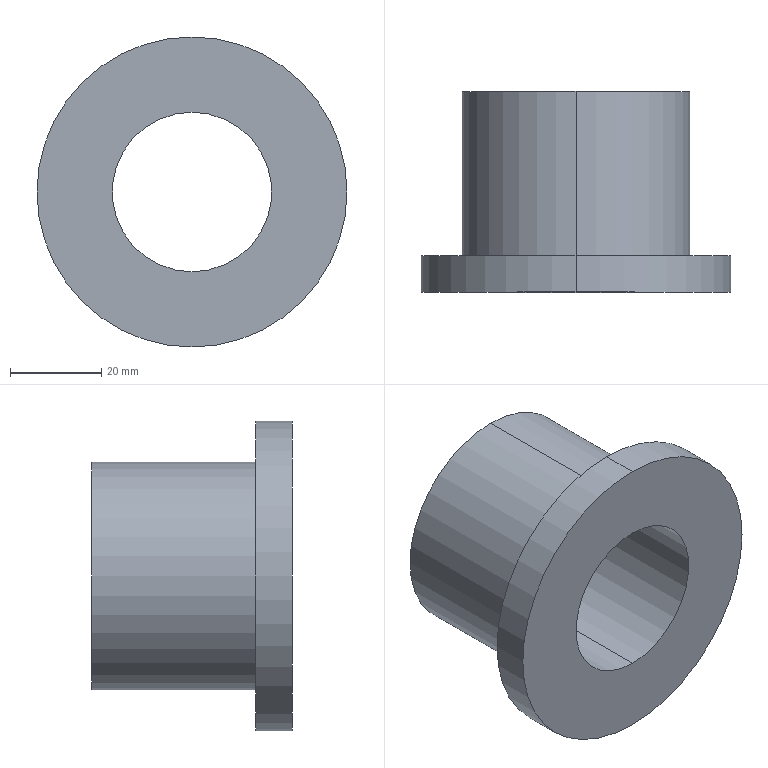Part | SolidWorks | features ICE 2, Extrusion 1 | 1 solid | 9 faces | box 68 x 44 x 68 mm | volume 57406 mm3 | cylinder 6 | plane 3 | commonest cylinder face diameters 35 x2 50 x2 68 x2
STEP:
#1=CARTESIAN_POINT('',(0.,0.,-17.5));
#2=VERTEX_POINT('',#1);
#3=CARTESIAN_POINT('',(0.,0.,17.5));
#4=VERTEX_POINT('',#3);
#5=CARTESIAN_POINT('',(0.,0.,0.));
#6=DIRECTION('',(0.,1.,0.));
#7=DIRECTION('',(0.,0.,1.));
#8=AXIS2_PLACEMENT_3D('',#5,#6,#7);
#9=CIRCLE('',#8,17.5);
#10=EDGE_CURVE('',#2,#4,#9,.T.);
#11=ORIENTED_EDGE('',*,*,#10,.F.);
#12=CARTESIAN_POINT('',(0.,44.,-17.5));
#13=VERTEX_POINT('',#12);
#14=CARTESIAN_POINT('',(0.,0.,-17.5));
#15=DIRECTION('',(0.,1.,0.));
#16=VECTOR('',#15,1000.);
#17=LINE('',#14,#16);
#18=EDGE_CURVE('',#2,#13,#17,.T.);
#19=ORIENTED_EDGE('',*,*,#18,.T.);
#20=CARTESIAN_POINT('',(0.,44.,17.5));
#21=VERTEX_POINT('',#20);
#22=CARTESIAN_POINT('',(0.,44.,0.));
#23=DIRECTION('',(0.,1.,0.));
#24=DIRECTION('',(0.,0.,1.));
#25=AXIS2_PLACEMENT_3D('',#22,#23,#24);
#26=CIRCLE('',#25,17.5);
#27=EDGE_CURVE('',#13,#21,#26,.T.);
#28=ORIENTED_EDGE('',*,*,#27,.T.);
#29=CARTESIAN_POINT('',(0.,0.,17.5));
#30=DIRECTION('',(0.,1.,0.));
#31=VECTOR('',#30,1000.);
#32=LINE('',#29,#31);
#33=EDGE_CURVE('',#4,#21,#32,.T.);
#34=ORIENTED_EDGE('',*,*,#33,.F.);
#35=EDGE_LOOP('',(#11,#19,#28,#34));
#36=FACE_OUTER_BOUND('',#35,.T.);
#37=CARTESIAN_POINT('',(0.,0.,0.));
#38=DIRECTION('',(0.,1.,0.));
#39=DIRECTION('',(0.,0.,1.));
#40=AXIS2_PLACEMENT_3D('',#37,#38,#39);
#41=CYLINDRICAL_SURFACE('',#40,17.5);
#42=ADVANCED_FACE('',(#36),#41,.F.);
#43=CARTESIAN_POINT('',(0.,44.,25.));
#44=VERTEX_POINT('',#43);
#45=CARTESIAN_POINT('',(0.,44.,-25.));
#46=VERTEX_POINT('',#45);
#47=CARTESIAN_POINT('',(0.,44.,0.));
#48=DIRECTION('',(0.,1.,0.));
#49=DIRECTION('',(0.,0.,1.));
#50=AXIS2_PLACEMENT_3D('',#47,#48,#49);
#51=CIRCLE('',#50,25.);
#52=EDGE_CURVE('',#44,#46,#51,.T.);
#53=ORIENTED_EDGE('',*,*,#52,.F.);
#54=CARTESIAN_POINT('',(0.,8.,25.));
#55=VERTEX_POINT('',#54);
#56=CARTESIAN_POINT('',(0.,44.,25.));
#57=DIRECTION('',(0.,-1.,0.));
#58=VECTOR('',#57,1000.);
#59=LINE('',#56,#58);
#60=EDGE_CURVE('',#44,#55,#59,.T.);
#61=ORIENTED_EDGE('',*,*,#60,.T.);
#62=CARTESIAN_POINT('',(0.,8.,-25.));
#63=VERTEX_POINT('',#62);
#64=CARTESIAN_POINT('',(0.,8.,0.));
#65=DIRECTION('',(0.,1.,0.));
#66=DIRECTION('',(0.,0.,1.));
#67=AXIS2_PLACEMENT_3D('',#64,#65,#66);
#68=CIRCLE('',#67,25.);
#69=EDGE_CURVE('',#55,#63,#68,.T.);
#70=ORIENTED_EDGE('',*,*,#69,.T.);
#71=CARTESIAN_POINT('',(0.,44.,-25.));
#72=DIRECTION('',(0.,-1.,0.));
#73=VECTOR('',#72,1000.);
#74=LINE('',#71,#73);
#75=EDGE_CURVE('',#46,#63,#74,.T.);
#76=ORIENTED_EDGE('',*,*,#75,.F.);
#77=EDGE_LOOP('',(#53,#61,#70,#76));
#78=FACE_OUTER_BOUND('',#77,.T.);
#79=CARTESIAN_POINT('',(0.,44.,0.));
#80=DIRECTION('',(0.,-1.,0.));
#81=DIRECTION('',(0.,0.,-1.));
#82=AXIS2_PLACEMENT_3D('',#79,#80,#81);
#83=CYLINDRICAL_SURFACE('',#82,25.);
#84=ADVANCED_FACE('',(#78),#83,.T.);
#85=CARTESIAN_POINT('',(0.,8.,34.));
#86=VERTEX_POINT('',#85);
#87=CARTESIAN_POINT('',(0.,8.,-34.));
#88=VERTEX_POINT('',#87);
#89=CARTESIAN_POINT('',(0.,8.,0.));
#90=DIRECTION('',(0.,1.,0.));
#91=DIRECTION('',(0.,0.,1.));
#92=AXIS2_PLACEMENT_3D('',#89,#90,#91);
#93=CIRCLE('',#92,34.);
#94=EDGE_CURVE('',#86,#88,#93,.T.);
#95=ORIENTED_EDGE('',*,*,#94,.F.);
#96=CARTESIAN_POINT('',(0.,0.,34.));
#97=VERTEX_POINT('',#96);
#98=CARTESIAN_POINT('',(0.,8.,34.));
#99=DIRECTION('',(0.,-1.,0.));
#100=VECTOR('',#99,1000.);
#101=LINE('',#98,#100);
#102=EDGE_CURVE('',#86,#97,#101,.T.);
#103=ORIENTED_EDGE('',*,*,#102,.T.);
#104=CARTESIAN_POINT('',(0.,0.,-34.));
#105=VERTEX_POINT('',#104);
#106=CARTESIAN_POINT('',(0.,0.,0.));
#107=DIRECTION('',(0.,1.,0.));
#108=DIRECTION('',(0.,0.,1.));
#109=AXIS2_PLACEMENT_3D('',#106,#107,#108);
#110=CIRCLE('',#109,34.);
#111=EDGE_CURVE('',#97,#105,#110,.T.);
#112=ORIENTED_EDGE('',*,*,#111,.T.);
#113=CARTESIAN_POINT('',(0.,8.,-34.));
#114=DIRECTION('',(0.,-1.,0.));
#115=VECTOR('',#114,1000.);
#116=LINE('',#113,#115);
#117=EDGE_CURVE('',#88,#105,#116,.T.);
#118=ORIENTED_EDGE('',*,*,#117,.F.);
#119=EDGE_LOOP('',(#95,#103,#112,#118));
#120=FACE_OUTER_BOUND('',#119,.T.);
#121=CARTESIAN_POINT('',(0.,8.,0.));
#122=DIRECTION('',(0.,-1.,0.));
#123=DIRECTION('',(0.,0.,-1.));
#124=AXIS2_PLACEMENT_3D('',#121,#122,#123);
#125=CYLINDRICAL_SURFACE('',#124,34.);
#126=ADVANCED_FACE('',(#120),#125,.T.);
#127=CARTESIAN_POINT('',(0.,8.,0.));
#128=DIRECTION('',(0.,1.,0.));
#129=DIRECTION('',(0.,0.,1.));
#130=AXIS2_PLACEMENT_3D('',#127,#128,#129);
#131=CIRCLE('',#130,34.);
#132=EDGE_CURVE('',#88,#86,#131,.T.);
#133=ORIENTED_EDGE('',*,*,#132,.T.);
#134=ORIENTED_EDGE('',*,*,#94,.T.);
#135=EDGE_LOOP('',(#133,#134));
#136=FACE_OUTER_BOUND('',#135,.T.);
#137=CARTESIAN_POINT('',(0.,8.,0.));
#138=DIRECTION('',(0.,1.,0.));
#139=DIRECTION('',(0.,0.,1.));
#140=AXIS2_PLACEMENT_3D('',#137,#138,#139);
#141=CIRCLE('',#140,25.);
#142=EDGE_CURVE('',#63,#55,#141,.T.);
#143=ORIENTED_EDGE('',*,*,#142,.F.);
#144=ORIENTED_EDGE('',*,*,#69,.F.);
#145=EDGE_LOOP('',(#143,#144));
#146=FACE_BOUND('',#145,.T.);
#147=CARTESIAN_POINT('',(0.,8.,0.));
#148=DIRECTION('',(0.,1.,0.));
#149=DIRECTION('',(0.,0.,1.));
#150=AXIS2_PLACEMENT_3D('',#147,#148,#149);
#151=PLANE('',#150);
#152=ADVANCED_FACE('',(#136,#146),#151,.T.);
#153=ORIENTED_EDGE('',*,*,#102,.F.);
#154=ORIENTED_EDGE('',*,*,#132,.F.);
#155=ORIENTED_EDGE('',*,*,#117,.T.);
#156=CARTESIAN_POINT('',(0.,0.,0.));
#157=DIRECTION('',(0.,1.,0.));
#158=DIRECTION('',(0.,0.,1.));
#159=AXIS2_PLACEMENT_3D('',#156,#157,#158);
#160=CIRCLE('',#159,34.);
#161=EDGE_CURVE('',#105,#97,#160,.T.);
#162=ORIENTED_EDGE('',*,*,#161,.T.);
#163=EDGE_LOOP('',(#153,#154,#155,#162));
#164=FACE_OUTER_BOUND('',#163,.T.);
#165=CARTESIAN_POINT('',(0.,8.,0.));
#166=DIRECTION('',(0.,-1.,0.));
#167=DIRECTION('',(0.,0.,-1.));
#168=AXIS2_PLACEMENT_3D('',#165,#166,#167);
#169=CYLINDRICAL_SURFACE('',#168,34.);
#170=ADVANCED_FACE('',(#164),#169,.T.);
#171=CARTESIAN_POINT('',(0.,0.,0.));
#172=DIRECTION('',(0.,1.,0.));
#173=DIRECTION('',(0.,0.,1.));
#174=AXIS2_PLACEMENT_3D('',#171,#172,#173);
#175=CIRCLE('',#174,17.5);
#176=EDGE_CURVE('',#4,#2,#175,.T.);
#177=ORIENTED_EDGE('',*,*,#176,.T.);
#178=ORIENTED_EDGE('',*,*,#10,.T.);
#179=EDGE_LOOP('',(#177,#178));
#180=FACE_BOUND('',#179,.T.);
#181=ORIENTED_EDGE('',*,*,#161,.F.);
#182=ORIENTED_EDGE('',*,*,#111,.F.);
#183=EDGE_LOOP('',(#181,#182));
#184=FACE_OUTER_BOUND('',#183,.T.);
#185=CARTESIAN_POINT('',(0.,0.,0.));
#186=DIRECTION('',(0.,1.,0.));
#187=DIRECTION('',(0.,0.,1.));
#188=AXIS2_PLACEMENT_3D('',#185,#186,#187);
#189=PLANE('',#188);
#190=ADVANCED_FACE('',(#180,#184),#189,.F.);
#191=ORIENTED_EDGE('',*,*,#60,.F.);
#192=CARTESIAN_POINT('',(0.,44.,0.));
#193=DIRECTION('',(0.,1.,0.));
#194=DIRECTION('',(0.,0.,1.));
#195=AXIS2_PLACEMENT_3D('',#192,#193,#194);
#196=CIRCLE('',#195,25.);
#197=EDGE_CURVE('',#46,#44,#196,.T.);
#198=ORIENTED_EDGE('',*,*,#197,.F.);
#199=ORIENTED_EDGE('',*,*,#75,.T.);
#200=ORIENTED_EDGE('',*,*,#142,.T.);
#201=EDGE_LOOP('',(#191,#198,#199,#200));
#202=FACE_OUTER_BOUND('',#201,.T.);
#203=CARTESIAN_POINT('',(0.,44.,0.));
#204=DIRECTION('',(0.,-1.,0.));
#205=DIRECTION('',(0.,0.,-1.));
#206=AXIS2_PLACEMENT_3D('',#203,#204,#205);
#207=CYLINDRICAL_SURFACE('',#206,25.);
#208=ADVANCED_FACE('',(#202),#207,.T.);
#209=CARTESIAN_POINT('',(0.,44.,0.));
#210=DIRECTION('',(0.,1.,0.));
#211=DIRECTION('',(0.,0.,1.));
#212=AXIS2_PLACEMENT_3D('',#209,#210,#211);
#213=CIRCLE('',#212,17.5);
#214=EDGE_CURVE('',#21,#13,#213,.T.);
#215=ORIENTED_EDGE('',*,*,#214,.F.);
#216=ORIENTED_EDGE('',*,*,#27,.F.);
#217=EDGE_LOOP('',(#215,#216));
#218=FACE_BOUND('',#217,.T.);
#219=ORIENTED_EDGE('',*,*,#197,.T.);
#220=ORIENTED_EDGE('',*,*,#52,.T.);
#221=EDGE_LOOP('',(#219,#220));
#222=FACE_OUTER_BOUND('',#221,.T.);
#223=CARTESIAN_POINT('',(0.,44.,0.));
#224=DIRECTION('',(0.,1.,0.));
#225=DIRECTION('',(0.,0.,1.));
#226=AXIS2_PLACEMENT_3D('',#223,#224,#225);
#227=PLANE('',#226);
#228=ADVANCED_FACE('',(#218,#222),#227,.T.);
#229=ORIENTED_EDGE('',*,*,#18,.F.);
#230=ORIENTED_EDGE('',*,*,#176,.F.);
#231=ORIENTED_EDGE('',*,*,#33,.T.);
#232=ORIENTED_EDGE('',*,*,#214,.T.);
#233=EDGE_LOOP('',(#229,#230,#231,#232));
#234=FACE_OUTER_BOUND('',#233,.T.);
#235=CARTESIAN_POINT('',(0.,0.,0.));
#236=DIRECTION('',(0.,1.,0.));
#237=DIRECTION('',(0.,0.,1.));
#238=AXIS2_PLACEMENT_3D('',#235,#236,#237);
#239=CYLINDRICAL_SURFACE('',#238,17.5);
#240=ADVANCED_FACE('',(#234),#239,.F.);
#241=CLOSED_SHELL('',(#42,#84,#126,#152,#170,#190,#208,#228,#240));
#242=MANIFOLD_SOLID_BREP('',#241);
#243=CARTESIAN_POINT('',(0.,0.,0.));
#244=DIRECTION('',(0.,0.,1.));
#245=DIRECTION('',(1.,0.,0.));
#246=AXIS2_PLACEMENT_3D('',#243,#244,#245);
#247=(LENGTH_UNIT()NAMED_UNIT(*)SI_UNIT(.MILLI.,.METRE.));
#248=UNCERTAINTY_MEASURE_WITH_UNIT(LENGTH_MEASURE(0.00001),#247,'','');
#249=(NAMED_UNIT(*)PLANE_ANGLE_UNIT()SI_UNIT($,.RADIAN.));
#250=(NAMED_UNIT(*)SI_UNIT($,.STERADIAN.)SOLID_ANGLE_UNIT());
#251=(GEOMETRIC_REPRESENTATION_CONTEXT(3)GLOBAL_UNCERTAINTY_ASSIGNED_CONTEXT((#248))GLOBAL_UNIT_ASSIGNED_CONTEXT((#247,#249,#250))REPRESENTATION_CONTEXT('',''));
#252=ADVANCED_BREP_SHAPE_REPRESENTATION('',(#242,#246),#251);